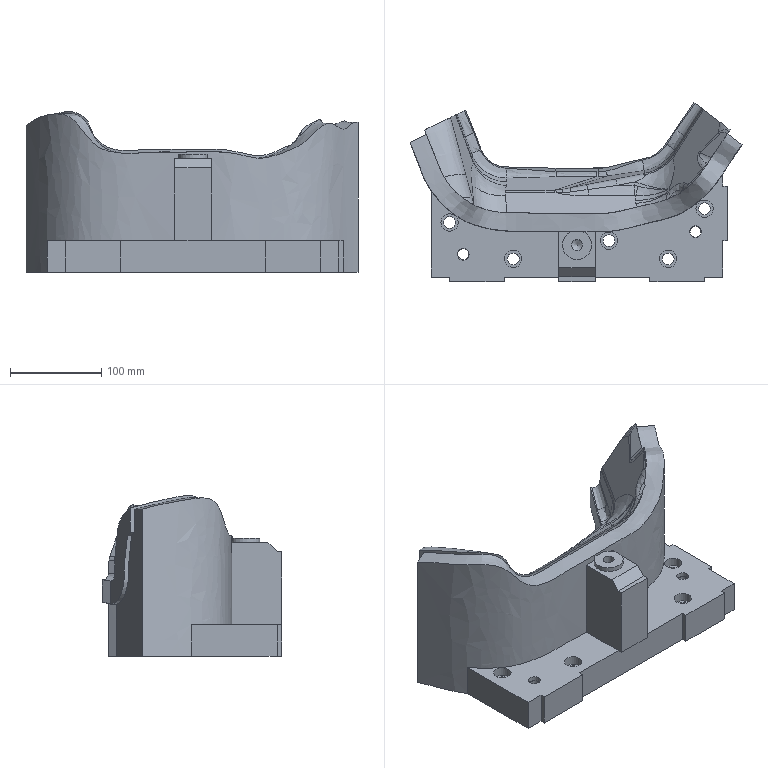Part | NX | features solid 2 | 1 solid | 143 faces | box 364.612 x 196.887 x 176.656 mm | volume 4224634 mm3 | spline 57 | plane 46 | cylinder 37 | sphere 2 | cone 1 | commonest cylinder face diameters 20 x12 13 x7 19 x5 12 x3 60 x3 100 x2